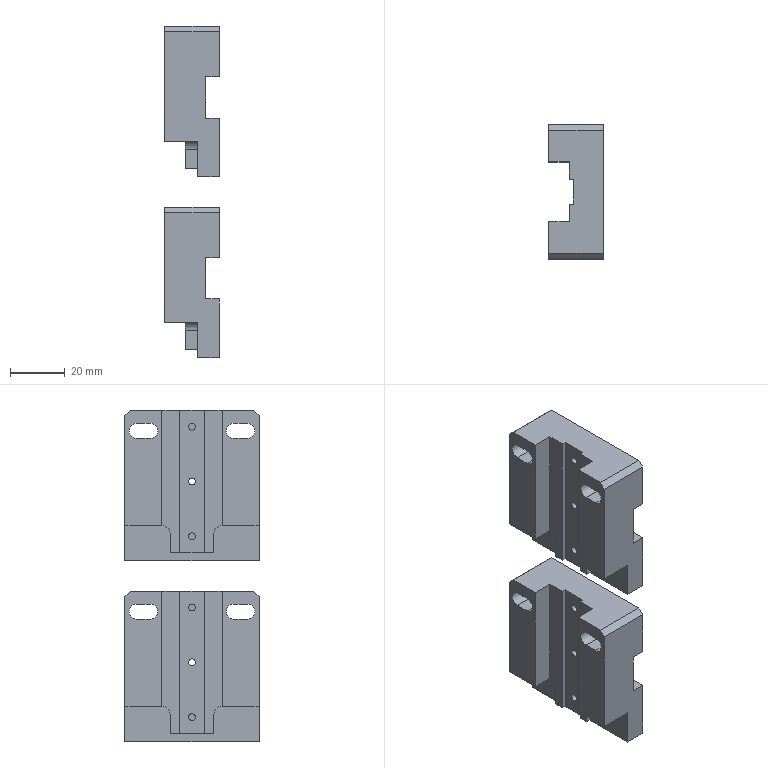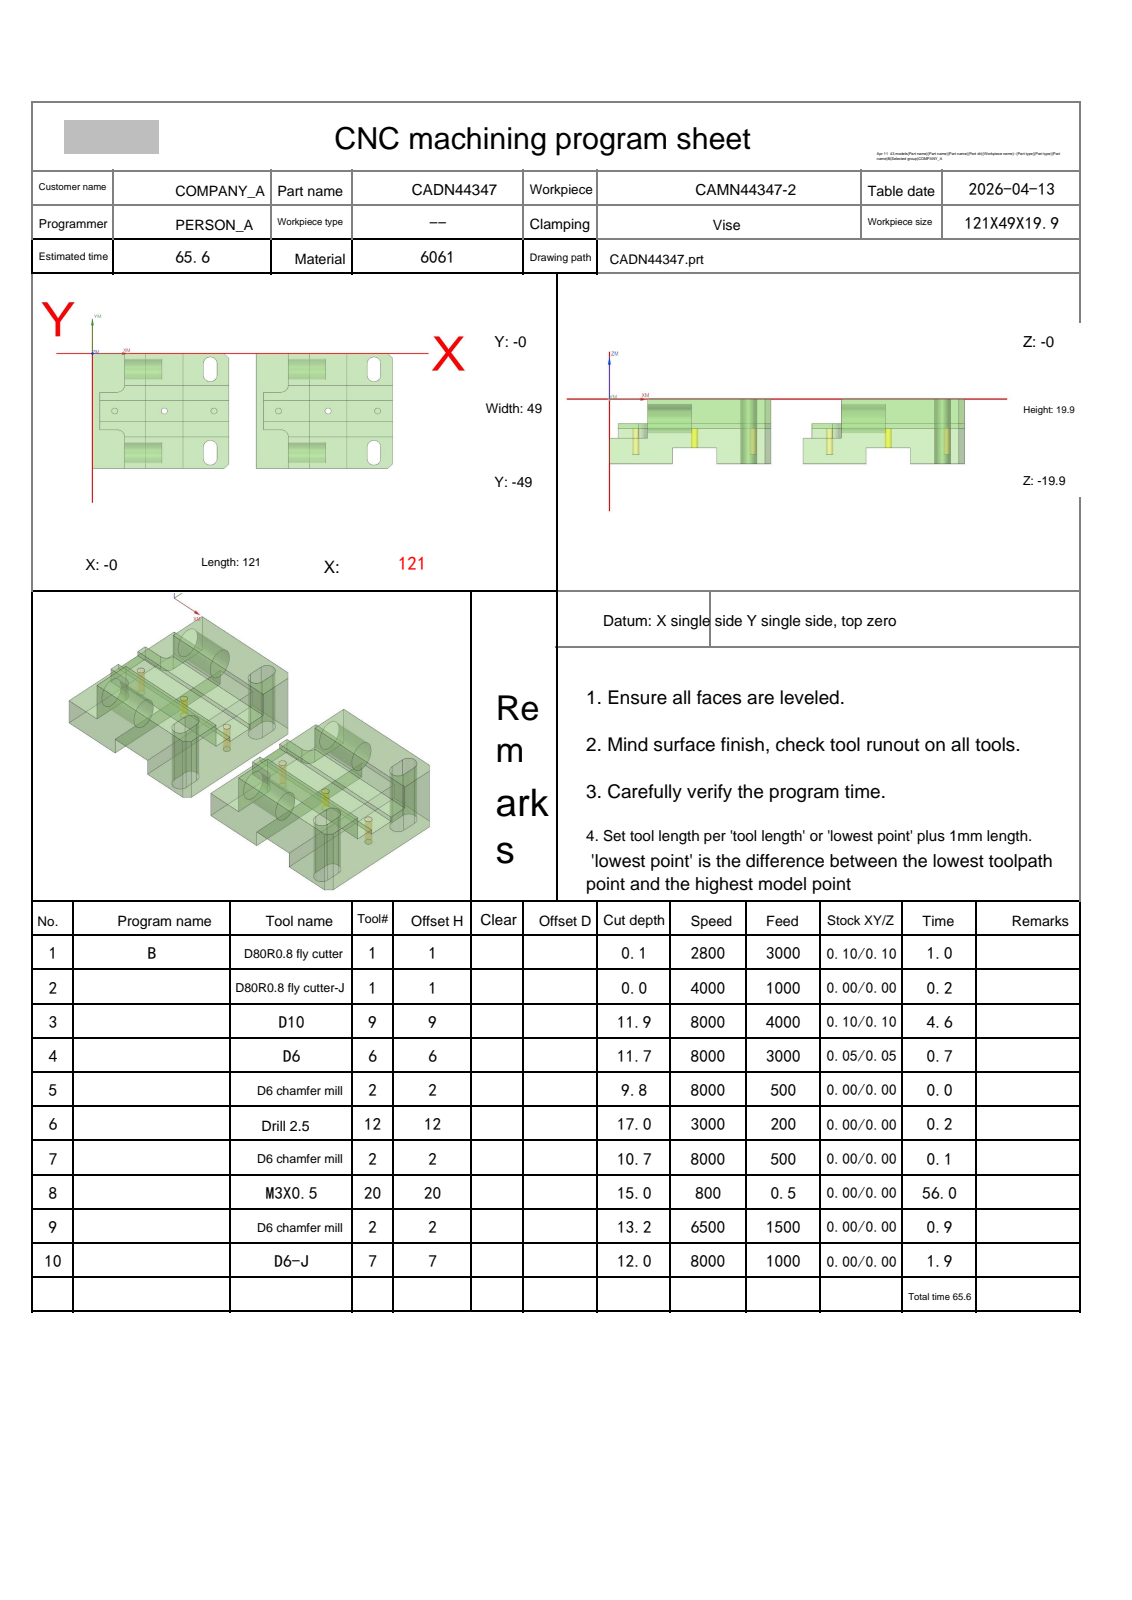NC program | NX | posted by the shop | part box 19.9 x 49 x 121 mm
Lines 120 to 1531 of 6263:
N3 T09 M06
(D10  D=10. R=0. H=09 ce=0.10 di=0.10)
G00 G90 G54 X67.5 Y-57. M03 S8000
G43 H09 Z14.902
M08
Z.905
G01 Z-.595 F4000.
Y-53.9
X61.1
Y4.9
X73.9
Y-11.4
X66.598
G02 X65.598 Y-10.4 I0.0 J1.
X65.64 Y-10.114 I1. J0.0
G01 X66.339 Y-7.77
G03 X66.38 Y-7.485 I-.958 J.285
X65.99 Y-6.693 I-1. J0.0
G02 X65.6 Y-5.902 I.61 J.793
G01 Y-.598
G02 X66.598 Y.4 I1. J-.002
G01 X68.402
G02 X69.4 Y-.598 I-.002 J-1.
G01 Y-5.902
G02 X69.038 Y-6.67 I-1. J.002
G03 X68.726 Y-7.128 I.638 J-.77
G01 X67.548 Y-10.712
G02 X66.598 Y-11.4 I-.95 J.312
G01 X63.9
Y-37.6
X73.9
Y-53.9
X70.27
G02 X69.451 Y-53.474 I0.0 J1.
G01 X66.836 Y-49.739
G03 X66.309 Y-49.357 I-.819 J-.574
G02 X65.6 Y-48.402 I.291 J.957
G01 Y-43.098
G02 X66.598 Y-42.1 I1. J-.002
G01 X68.402
G02 X69.4 Y-43.098 I-.002 J-1.
G01 Y-48.402
G02 X68.402 Y-49.4 I-1. J.002
G01 X67.5
X67.
Y-57.
Z.905
G00 X67.5
Z.31
G01 Z-1.19
Y-53.9
X61.1
Y4.9
X73.9
Y-11.4
X66.598
G02 X65.598 Y-10.4 I0.0 J1.
X65.64 Y-10.114 I1. J0.0
G01 X66.339 Y-7.77
G03 X66.38 Y-7.485 I-.958 J.285
X65.99 Y-6.693 I-1. J0.0
G02 X65.6 Y-5.902 I.61 J.793
G01 Y-.598
G02 X66.598 Y.4 I1. J-.002
G01 X68.402
G02 X69.4 Y-.598 I-.002 J-1.
G01 Y-5.902
G02 X69.038 Y-6.67 I-1. J.002
G03 X68.726 Y-7.128 I.638 J-.77
G01 X67.548 Y-10.712
G02 X66.598 Y-11.4 I-.95 J.312
G01 X63.9
Y-37.6
X73.9
Y-53.9
X70.27
G02 X69.451 Y-53.474 I0.0 J1.
G01 X66.836 Y-49.739
G03 X66.309 Y-49.357 I-.819 J-.574
G02 X65.6 Y-48.402 I.291 J.957
G01 Y-43.098
G02 X66.598 Y-42.1 I1. J-.002
G01 X68.402
G02 X69.4 Y-43.098 I-.002 J-1.
G01 Y-48.402
G02 X68.402 Y-49.4 I-1. J.002
G01 X67.5
X67.
Y-57.
Z.31
G00 X67.5
Z-.285
G01 Z-1.785
Y-53.9
X61.1
Y4.9
X73.9
Y-11.4
X66.598
G02 X65.598 Y-10.4 I0.0 J1.
X65.64 Y-10.114 I1. J0.0
G01 X66.339 Y-7.77
G03 X66.38 Y-7.485 I-.958 J.285
X65.99 Y-6.693 I-1. J0.0
G02 X65.6 Y-5.902 I.61 J.793
G01 Y-.598
G02 X66.598 Y.4 I1. J-.002
G01 X68.402
G02 X69.4 Y-.598 I-.002 J-1.
G01 Y-5.902
G02 X69.038 Y-6.67 I-1. J.002
G03 X68.726 Y-7.128 I.638 J-.77
G01 X67.548 Y-10.712
G02 X66.598 Y-11.4 I-.95 J.312
G01 X63.9
Y-37.6
X73.9
Y-53.9
X70.27
G02 X69.451 Y-53.474 I0.0 J1.
G01 X66.836 Y-49.739
G03 X66.309 Y-49.357 I-.819 J-.574
G02 X65.6 Y-48.402 I.291 J.957
G01 Y-43.098
G02 X66.598 Y-42.1 I1. J-.002
G01 X68.402
G02 X69.4 Y-43.098 I-.002 J-1.
G01 Y-48.402
G02 X68.402 Y-49.4 I-1. J.002
G01 X67.5
X67.
Y-57.
Z-.285
G00 X67.5
Z-.88
G01 Z-2.38
Y-53.9
X61.1
Y4.9
X73.9
Y-11.4
X66.598
G02 X65.598 Y-10.4 I0.0 J1.
X65.64 Y-10.114 I1. J0.0
G01 X66.339 Y-7.77
G03 X66.38 Y-7.485 I-.958 J.285
X65.99 Y-6.693 I-1. J0.0
G02 X65.6 Y-5.902 I.61 J.793
G01 Y-.598
G02 X66.598 Y.4 I1. J-.002
G01 X68.402
G02 X69.4 Y-.598 I-.002 J-1.
G01 Y-5.902
G02 X69.038 Y-6.67 I-1. J.002
G03 X68.726 Y-7.128 I.638 J-.77
G01 X67.548 Y-10.712
G02 X66.598 Y-11.4 I-.95 J.312
G01 X63.9
Y-37.6
X73.9
Y-53.9
X70.27
G02 X69.451 Y-53.474 I0.0 J1.
G01 X66.836 Y-49.739
G03 X66.309 Y-49.357 I-.819 J-.574
G02 X65.6 Y-48.402 I.291 J.957
G01 Y-43.098
G02 X66.598 Y-42.1 I1. J-.002
G01 X68.402
G02 X69.4 Y-43.098 I-.002 J-1.
G01 Y-48.402
G02 X68.402 Y-49.4 I-1. J.002
G01 X67.5
X67.
Y-57.
Z-.88
G00 X67.5
Z-1.475
G01 Z-2.975
Y-53.9
X61.1
Y4.9
X73.9
Y-11.4
X66.598
G02 X65.598 Y-10.4 I0.0 J1.
X65.64 Y-10.114 I1. J0.0
G01 X66.339 Y-7.77
G03 X66.38 Y-7.485 I-.958 J.285
X65.99 Y-6.693 I-1. J0.0
G02 X65.6 Y-5.902 I.61 J.793
G01 Y-.598
G02 X66.598 Y.4 I1. J-.002
G01 X68.402
G02 X69.4 Y-.598 I-.002 J-1.
G01 Y-5.902
G02 X69.038 Y-6.67 I-1. J.002
G03 X68.726 Y-7.128 I.638 J-.77
G01 X67.548 Y-10.712
G02 X66.598 Y-11.4 I-.95 J.312
G01 X63.9
Y-37.6
X73.9
Y-53.9
X70.27
G02 X69.451 Y-53.474 I0.0 J1.
G01 X66.836 Y-49.739
G03 X66.309 Y-49.357 I-.819 J-.574
G02 X65.6 Y-48.402 I.291 J.957
G01 Y-43.098
G02 X66.598 Y-42.1 I1. J-.002
G01 X68.402
G02 X69.4 Y-43.098 I-.002 J-1.
G01 Y-48.402
G02 X68.402 Y-49.4 I-1. J.002
G01 X67.5
X67.
Y-57.
Z-1.475
G00 X67.5
Z-2.07
G01 Z-3.57
Y-53.9
X61.1
Y4.9
X73.9
Y-11.4
X66.598
G02 X65.598 Y-10.4 I0.0 J1.
X65.64 Y-10.114 I1. J0.0
G01 X66.339 Y-7.77
G03 X66.38 Y-7.485 I-.958 J.285
X65.99 Y-6.693 I-1. J0.0
G02 X65.6 Y-5.902 I.61 J.793
G01 Y-.598
G02 X66.598 Y.4 I1. J-.002
G01 X68.402
G02 X69.4 Y-.598 I-.002 J-1.
G01 Y-5.902
G02 X69.038 Y-6.67 I-1. J.002
G03 X68.726 Y-7.128 I.638 J-.77
G01 X67.548 Y-10.712
G02 X66.598 Y-11.4 I-.95 J.312
G01 X63.9
Y-37.6
X73.9
Y-53.9
X70.27
G02 X69.451 Y-53.474 I0.0 J1.
G01 X66.836 Y-49.739
G03 X66.309 Y-49.357 I-.819 J-.574
G02 X65.6 Y-48.402 I.291 J.957
G01 Y-43.098
G02 X66.598 Y-42.1 I1. J-.002
G01 X68.402
G02 X69.4 Y-43.098 I-.002 J-1.
G01 Y-48.402
G02 X68.402 Y-49.4 I-1. J.002
G01 X67.5
X67.
Y-57.
Z-2.07
G00 X67.5
Z-2.665
G01 Z-4.165
Y-53.9
X61.1
Y4.9
X73.9
Y-11.4
X66.598
G02 X65.598 Y-10.4 I0.0 J1.
X65.64 Y-10.114 I1. J0.0
G01 X66.339 Y-7.77
G03 X66.38 Y-7.485 I-.958 J.285
X65.99 Y-6.693 I-1. J0.0
G02 X65.6 Y-5.902 I.61 J.793
G01 Y-.598
G02 X66.598 Y.4 I1. J-.002
G01 X68.402
G02 X69.4 Y-.598 I-.002 J-1.
G01 Y-5.902
G02 X69.038 Y-6.67 I-1. J.002
G03 X68.726 Y-7.128 I.638 J-.77
G01 X67.548 Y-10.712
G02 X66.598 Y-11.4 I-.95 J.312
G01 X63.9
Y-37.6
X73.9
Y-53.9
X70.27
G02 X69.451 Y-53.474 I0.0 J1.
G01 X66.836 Y-49.739
G03 X66.309 Y-49.357 I-.819 J-.574
G02 X65.6 Y-48.402 I.291 J.957
G01 Y-43.098
G02 X66.598 Y-42.1 I1. J-.002
G01 X68.402
G02 X69.4 Y-43.098 I-.002 J-1.
G01 Y-48.402
G02 X68.402 Y-49.4 I-1. J.002
G01 X67.5
X67.
Y-57.
Z-2.665
G00 X67.5
Z-3.26
G01 Z-4.76
Y-53.9
X61.1
Y4.9
X73.9
Y-11.4
X66.598
G02 X65.598 Y-10.4 I0.0 J1.
X65.64 Y-10.114 I1. J0.0
G01 X66.339 Y-7.77
G03 X66.38 Y-7.485 I-.958 J.285
X65.99 Y-6.693 I-1. J0.0
G02 X65.6 Y-5.902 I.61 J.793
G01 Y-.598
G02 X66.598 Y.4 I1. J-.002
G01 X68.402
G02 X69.4 Y-.598 I-.002 J-1.
G01 Y-5.902
G02 X69.038 Y-6.67 I-1. J.002
G03 X68.726 Y-7.128 I.638 J-.77
G01 X67.548 Y-10.712
G02 X66.598 Y-11.4 I-.95 J.312
G01 X63.9
Y-37.6
X73.9
Y-53.9
X70.27
G02 X69.451 Y-53.474 I0.0 J1.
G01 X66.836 Y-49.739
G03 X66.309 Y-49.357 I-.819 J-.574
G02 X65.6 Y-48.402 I.291 J.957
G01 Y-43.098
G02 X66.598 Y-42.1 I1. J-.002
G01 X68.402
G02 X69.4 Y-43.098 I-.002 J-1.
G01 Y-48.402
G02 X68.402 Y-49.4 I-1. J.002
G01 X67.5
X67.
Y-57.
Z-3.26
G00 X67.5
Z-3.855
G01 Z-5.355
Y-53.9
X61.1
Y4.9
X73.9
Y-11.4
X66.598
G02 X65.598 Y-10.4 I0.0 J1.
X65.64 Y-10.114 I1. J0.0
G01 X66.339 Y-7.77
G03 X66.38 Y-7.485 I-.958 J.285
X65.99 Y-6.693 I-1. J0.0
G02 X65.6 Y-5.902 I.61 J.793
G01 Y-.598
G02 X66.598 Y.4 I1. J-.002
G01 X68.402
G02 X69.4 Y-.598 I-.002 J-1.
G01 Y-5.902
G02 X69.038 Y-6.67 I-1. J.002
G03 X68.726 Y-7.128 I.638 J-.77
G01 X67.548 Y-10.712
G02 X66.598 Y-11.4 I-.95 J.312
G01 X63.9
Y-37.6
X73.9
Y-53.9
X70.27
G02 X69.451 Y-53.474 I0.0 J1.
G01 X66.836 Y-49.739
G03 X66.309 Y-49.357 I-.819 J-.574
G02 X65.6 Y-48.402 I.291 J.957
G01 Y-43.098
G02 X66.598 Y-42.1 I1. J-.002
G01 X68.402
G02 X69.4 Y-43.098 I-.002 J-1.
G01 Y-48.402
G02 X68.402 Y-49.4 I-1. J.002
G01 X67.5
X67.
Y-57.
Z-3.855
G00 X67.5
Z-4.45
G01 Z-5.95
Y-53.9
X61.1
Y4.9
X73.9
Y-11.4
X66.598
G02 X65.598 Y-10.4 I0.0 J1.
X65.64 Y-10.114 I1. J0.0
G01 X66.339 Y-7.77
G03 X66.38 Y-7.485 I-.958 J.285
X65.99 Y-6.693 I-1. J0.0
G02 X65.6 Y-5.902 I.61 J.793
G01 Y-.598
G02 X66.598 Y.4 I1. J-.002
G01 X68.402
G02 X69.4 Y-.598 I-.002 J-1.
G01 Y-5.902
G02 X69.038 Y-6.67 I-1. J.002
G03 X68.726 Y-7.128 I.638 J-.77
G01 X67.548 Y-10.712
G02 X66.598 Y-11.4 I-.95 J.312
G01 X63.9
Y-37.6
X73.9
Y-53.9
X70.27
G02 X69.451 Y-53.474 I0.0 J1.
G01 X66.836 Y-49.739
G03 X66.309 Y-49.357 I-.819 J-.574
G02 X65.6 Y-48.402 I.291 J.957
G01 Y-43.098
G02 X66.598 Y-42.1 I1. J-.002
G01 X68.402
G02 X69.4 Y-43.098 I-.002 J-1.
G01 Y-48.402
G02 X68.402 Y-49.4 I-1. J.002
G01 X67.5
X67.
Y-57.
Z-4.45
G00 X67.5
Z-5.045
G01 Z-6.545
Y-53.9
X61.1
Y4.9
X73.9
Y-11.4
X66.598
G02 X65.598 Y-10.4 I0.0 J1.
X65.64 Y-10.114 I1. J0.0
G01 X66.339 Y-7.77
G03 X66.38 Y-7.485 I-.958 J.285
X65.99 Y-6.693 I-1. J0.0
G02 X65.6 Y-5.902 I.61 J.793
G01 Y-.598
G02 X66.598 Y.4 I1. J-.002
G01 X68.402
G02 X69.4 Y-.598 I-.002 J-1.
G01 Y-5.902
G02 X69.038 Y-6.67 I-1. J.002
G03 X68.726 Y-7.128 I.638 J-.77
G01 X67.548 Y-10.712
G02 X66.598 Y-11.4 I-.95 J.312
G01 X63.9
Y-37.6
X73.9
Y-53.9
X70.27
G02 X69.451 Y-53.474 I0.0 J1.
G01 X66.836 Y-49.739
G03 X66.309 Y-49.357 I-.819 J-.574
G02 X65.6 Y-48.402 I.291 J.957
G01 Y-43.098
G02 X66.598 Y-42.1 I1. J-.002
G01 X68.402
G02 X69.4 Y-43.098 I-.002 J-1.
G01 Y-48.402
G02 X68.402 Y-49.4 I-1. J.002
G01 X67.5
X67.
Y-57.
Z-5.045
G00 X67.5
Z-5.64
G01 Z-7.14
Y-53.9
X61.1
Y4.9
X73.9
Y-11.4
X66.598
G02 X65.598 Y-10.4 I0.0 J1.
X65.64 Y-10.114 I1. J0.0
G01 X66.339 Y-7.77
G03 X66.38 Y-7.485 I-.958 J.285
X65.99 Y-6.693 I-1. J0.0
G02 X65.6 Y-5.902 I.61 J.793
G01 Y-.598
G02 X66.598 Y.4 I1. J-.002
G01 X68.402
G02 X69.4 Y-.598 I-.002 J-1.
G01 Y-5.902
G02 X69.038 Y-6.67 I-1. J.002
G03 X68.726 Y-7.128 I.638 J-.77
G01 X67.548 Y-10.712
G02 X66.598 Y-11.4 I-.95 J.312
G01 X63.9
Y-37.6
X73.9
Y-53.9
X70.27
G02 X69.451 Y-53.474 I0.0 J1.
G01 X66.836 Y-49.739
G03 X66.309 Y-49.357 I-.819 J-.574
G02 X65.6 Y-48.402 I.291 J.957
G01 Y-43.098
G02 X66.598 Y-42.1 I1. J-.002
G01 X68.402
G02 X69.4 Y-43.098 I-.002 J-1.
G01 Y-48.402
G02 X68.402 Y-49.4 I-1. J.002
G01 X67.5
X67.
Y-57.
Z-5.64
G00 X67.5
Z-6.235
G01 Z-7.735
Y-53.9
X61.1
Y4.9
X73.9
Y-11.4
X66.598
G02 X65.598 Y-10.4 I0.0 J1.
X65.64 Y-10.114 I1. J0.0
G01 X66.339 Y-7.77
G03 X66.38 Y-7.485 I-.958 J.285
X65.99 Y-6.693 I-1. J0.0
G02 X65.6 Y-5.902 I.61 J.793
G01 Y-.598
G02 X66.598 Y.4 I1. J-.002
G01 X68.402
G02 X69.4 Y-.598 I-.002 J-1.
G01 Y-5.902
G02 X69.038 Y-6.67 I-1. J.002
G03 X68.726 Y-7.128 I.638 J-.77
G01 X67.548 Y-10.712
G02 X66.598 Y-11.4 I-.95 J.312
G01 X63.9
Y-37.6
X73.9
Y-53.9
X70.27
G02 X69.451 Y-53.474 I0.0 J1.
G01 X66.836 Y-49.739
G03 X66.309 Y-49.357 I-.819 J-.574
G02 X65.6 Y-48.402 I.291 J.957
G01 Y-43.098
G02 X66.598 Y-42.1 I1. J-.002
G01 X68.402
G02 X69.4 Y-43.098 I-.002 J-1.
G01 Y-48.402
G02 X68.402 Y-49.4 I-1. J.002
G01 X67.5
X67.
Y-57.
Z-6.235
G00 X67.5
Z-6.83
G01 Z-8.33
Y-53.9
X61.1
Y4.9
X73.9
Y-11.4
X66.598
G02 X65.598 Y-10.4 I0.0 J1.
X65.64 Y-10.114 I1. J0.0
G01 X66.339 Y-7.77
G03 X66.38 Y-7.485 I-.958 J.285
X65.99 Y-6.693 I-1. J0.0
G02 X65.6 Y-5.902 I.61 J.793
G01 Y-.598
G02 X66.598 Y.4 I1. J-.002
G01 X68.402
G02 X69.4 Y-.598 I-.002 J-1.
G01 Y-5.902
G02 X69.038 Y-6.67 I-1. J.002
G03 X68.726 Y-7.128 I.638 J-.77
G01 X67.548 Y-10.712
G02 X66.598 Y-11.4 I-.95 J.312
G01 X63.9
Y-37.6
X73.9
Y-53.9
X70.27
G02 X69.451 Y-53.474 I0.0 J1.
G01 X66.836 Y-49.739
G03 X66.309 Y-49.357 I-.819 J-.574
G02 X65.6 Y-48.402 I.291 J.957
G01 Y-43.098
G02 X66.598 Y-42.1 I1. J-.002
G01 X68.402
G02 X69.4 Y-43.098 I-.002 J-1.
G01 Y-48.402
G02 X68.402 Y-49.4 I-1. J.002
G01 X67.5
X67.
Y-57.
Z-6.83
G00 X67.5
Z-7.425
G01 Z-8.925
Y-53.9
X61.1
Y4.9
X73.9
Y-11.4
X66.598
G02 X65.598 Y-10.4 I0.0 J1.
X65.64 Y-10.114 I1. J0.0
G01 X66.339 Y-7.77
G03 X66.38 Y-7.485 I-.958 J.285
X65.99 Y-6.693 I-1. J0.0
G02 X65.6 Y-5.902 I.61 J.793
G01 Y-.598
G02 X66.598 Y.4 I1. J-.002
G01 X68.402
G02 X69.4 Y-.598 I-.002 J-1.
G01 Y-5.902
G02 X69.038 Y-6.67 I-1. J.002
G03 X68.726 Y-7.128 I.638 J-.77
G01 X67.548 Y-10.712
G02 X66.598 Y-11.4 I-.95 J.312
G01 X63.9
Y-37.6
X73.9
Y-53.9
X70.27
G02 X69.451 Y-53.474 I0.0 J1.
G01 X66.836 Y-49.739
G03 X66.309 Y-49.357 I-.819 J-.574
G02 X65.6 Y-48.402 I.291 J.957
G01 Y-43.098
G02 X66.598 Y-42.1 I1. J-.002
G01 X68.402
G02 X69.4 Y-43.098 I-.002 J-1.
G01 Y-48.402
G02 X68.402 Y-49.4 I-1. J.002
G01 X67.5
X67.
Y-57.
Z-7.425
G00 X67.5
Z-8.02
G01 Z-9.52
Y-53.9
X61.1
Y4.9
X73.9
Y-11.4
X66.598
G02 X65.598 Y-10.4 I0.0 J1.
X65.64 Y-10.114 I1. J0.0
G01 X66.339 Y-7.77
G03 X66.38 Y-7.485 I-.958 J.285
X65.99 Y-6.693 I-1. J0.0
G02 X65.6 Y-5.902 I.61 J.793
G01 Y-.598
G02 X66.598 Y.4 I1. J-.002
G01 X68.402
G02 X69.4 Y-.598 I-.002 J-1.
G01 Y-5.902
G02 X69.038 Y-6.67 I-1. J.002
G03 X68.726 Y-7.128 I.638 J-.77
G01 X67.548 Y-10.712
G02 X66.598 Y-11.4 I-.95 J.312
G01 X63.9
Y-37.6
X73.9
Y-53.9
X70.27
G02 X69.451 Y-53.474 I0.0 J1.
G01 X66.836 Y-49.739
G03 X66.309 Y-49.357 I-.819 J-.574
G02 X65.6 Y-48.402 I.291 J.957
G01 Y-43.098
G02 X66.598 Y-42.1 I1. J-.002
G01 X68.402
G02 X69.4 Y-43.098 I-.002 J-1.
G01 Y-48.402
G02 X68.402 Y-49.4 I-1. J.002
G01 X67.5
X67.
Y-57.
Z-8.02
G00 X67.5
Z-8.615
G01 Z-10.115
Y-53.9
X61.1
Y4.9
X73.9
Y-11.4
X66.598
G02 X65.598 Y-10.4 I0.0 J1.
X65.64 Y-10.114 I1. J0.0
G01 X66.339 Y-7.77
G03 X66.38 Y-7.485 I-.958 J.285
X65.99 Y-6.693 I-1. J0.0
G02 X65.6 Y-5.902 I.61 J.793
G01 Y-.598
G02 X66.598 Y.4 I1. J-.002
G01 X68.402
G02 X69.4 Y-.598 I-.002 J-1.
G01 Y-5.902
G02 X69.038 Y-6.67 I-1. J.002
G03 X68.726 Y-7.128 I.638 J-.77
G01 X67.548 Y-10.712
G02 X66.598 Y-11.4 I-.95 J.312
G01 X63.9
Y-37.6
X73.9
Y-53.9
X70.27
G02 X69.451 Y-53.474 I0.0 J1.
G01 X66.836 Y-49.739
G03 X66.309 Y-49.357 I-.819 J-.574
G02 X65.6 Y-48.402 I.291 J.957
G01 Y-43.098
G02 X66.598 Y-42.1 I1. J-.002
G01 X68.402
G02 X69.4 Y-43.098 I-.002 J-1.
G01 Y-48.402
G02 X68.402 Y-49.4 I-1. J.002
G01 X67.5
X67.
Y-57.
Z-8.615
G00 X67.5
Z-9.21
G01 Z-10.71
Y-53.9
X61.1
Y4.9
X73.9
Y-11.4
X66.598
G02 X65.598 Y-10.4 I0.0 J1.
X65.64 Y-10.114 I1. J0.0
G01 X66.339 Y-7.77
G03 X66.38 Y-7.485 I-.958 J.285
X65.99 Y-6.693 I-1. J0.0
G02 X65.6 Y-5.902 I.61 J.793
G01 Y-.598
G02 X66.598 Y.4 I1. J-.002
G01 X68.402
G02 X69.4 Y-.598 I-.002 J-1.
G01 Y-5.902
G02 X69.038 Y-6.67 I-1. J.002
G03 X68.726 Y-7.128 I.638 J-.77
G01 X67.548 Y-10.712
G02 X66.598 Y-11.4 I-.95 J.312
G01 X63.9
Y-37.6
X73.9
Y-53.9
X70.27
G02 X69.451 Y-53.474 I0.0 J1.
G01 X66.836 Y-49.739
G03 X66.309 Y-49.357 I-.819 J-.574
G02 X65.6 Y-48.402 I.291 J.957
G01 Y-43.098
G02 X66.598 Y-42.1 I1. J-.002
G01 X68.402
G02 X69.4 Y-43.098 I-.002 J-1.
G01 Y-48.402
G02 X68.402 Y-49.4 I-1. J.002
G01 X67.5
X67.
Y-57.
Z-9.21
G00 X67.5
Z-9.805
G01 Z-11.305
Y-53.9
X61.1
Y4.9
X73.9
Y-11.4
X66.598
G02 X65.598 Y-10.4 I0.0 J1.
X65.64 Y-10.114 I1. J0.0
G01 X66.339 Y-7.77
G03 X66.38 Y-7.485 I-.958 J.285
X65.99 Y-6.693 I-1. J0.0
G02 X65.6 Y-5.902 I.61 J.793
G01 Y-.598
G02 X66.598 Y.4 I1. J-.002
G01 X68.402
G02 X69.4 Y-.598 I-.002 J-1.
G01 Y-5.902
G02 X69.038 Y-6.67 I-1. J.002
G03 X68.726 Y-7.128 I.638 J-.77
G01 X67.548 Y-10.712
G02 X66.598 Y-11.4 I-.95 J.312
G01 X63.9
Y-37.6
X73.9
Y-53.9
X70.27
G02 X69.451 Y-53.474 I0.0 J1.
G01 X66.836 Y-49.739
G03 X66.309 Y-49.357 I-.819 J-.574
G02 X65.6 Y-48.402 I.291 J.957
G01 Y-43.098
G02 X66.598 Y-42.1 I1. J-.002
G01 X68.402
G02 X69.4 Y-43.098 I-.002 J-1.
G01 Y-48.402
G02 X68.402 Y-49.4 I-1. J.002
G01 X67.5
X67.
Y-57.
Z-9.805
G00 X67.5
Z-10.4
G01 Z-11.9
Y-53.9
X61.1
Y4.9
X73.9
Y-11.4
X66.598
G02 X65.598 Y-10.4 I0.0 J1.
X65.64 Y-10.114 I1. J0.0
G01 X66.339 Y-7.77
G03 X66.38 Y-7.485 I-.958 J.285
X65.99 Y-6.693 I-1. J0.0
G02 X65.6 Y-5.902 I.61 J.793
G01 Y-.598
G02 X66.598 Y.4 I1. J-.002
G01 X68.402
G02 X69.4 Y-.598 I-.002 J-1.
G01 Y-5.902
G02 X69.038 Y-6.67 I-1. J.002
G03 X68.726 Y-7.128 I.638 J-.77
G01 X67.548 Y-10.712
G02 X66.598 Y-11.4 I-.95 J.312
G01 X63.9
Y-37.6
X73.9
Y-53.9
X70.27
G02 X69.451 Y-53.474 I0.0 J1.
G01 X66.836 Y-49.739
G03 X66.309 Y-49.357 I-.819 J-.574
G02 X65.6 Y-48.402 I.291 J.957
G01 Y-43.098
G02 X66.598 Y-42.1 I1. J-.002
G01 X68.402
G02 X69.4 Y-43.098 I-.002 J-1.
G01 Y-48.402
G02 X68.402 Y-49.4 I-1. J.002
G01 X67.5
X67.
Y-57.
Z-10.4
G00 Z14.902
X-8. Y-45.75
Z.905
G01 Z-.595
X-4.9
Y4.9
X7.9
Y-11.4
X.598
G02 X-.402 Y-10.4 I0.0 J1.
X-.36 Y-10.114 I1. J0.0
G01 X.339 Y-7.77
G03 X.38 Y-7.485 I-.958 J.285
X-.01 Y-6.693 I-1. J0.0
G02 X-.4 Y-5.902 I.61 J.793
G01 Y-.598
G02 X.598 Y.4 I1. J-.002
G01 X2.402
G02 X3.4 Y-.598 I-.002 J-1.
G01 Y-5.902
G02 X3.038 Y-6.67 I-1. J.002
G03 X2.726 Y-7.128 I.638 J-.77
G01 X1.548 Y-10.712
G02 X.598 Y-11.4 I-.95 J.312
G01 X-2.1
Y-37.6
X7.9
Y-53.9
X-4.9
Y-48.414
G02 X-4.607 Y-47.707 I1. J0.0
G01 X-.693 Y-43.793
G03 X-.4 Y-43.093 I-.707 J.707
G02 X.598 Y-42.1 I1. J-.007
G01 X2.402
G02 X3.4 Y-43.098 I-.002 J-1.
G01 Y-48.402
G02 X2.402 Y-49.4 I-1. J.002
G01 X.598
G02 X-.4 Y-48.402 I.002 J1.
G01 Y-45.75
Y-45.25
X-8.
Z.905
G00 Y-45.75
Z.31
G01 Z-1.19
X-4.9
Y4.9
X7.9
Y-11.4
X.598
G02 X-.402 Y-10.4 I0.0 J1.
X-.36 Y-10.114 I1. J0.0
G01 X.339 Y-7.77
G03 X.38 Y-7.485 I-.958 J.285
X-.01 Y-6.693 I-1. J0.0
G02 X-.4 Y-5.902 I.61 J.793
G01 Y-.598
G02 X.598 Y.4 I1. J-.002
G01 X2.402
G02 X3.4 Y-.598 I-.002 J-1.
G01 Y-5.902
G02 X3.038 Y-6.67 I-1. J.002
G03 X2.726 Y-7.128 I.638 J-.77
G01 X1.548 Y-10.712
G02 X.598 Y-11.4 I-.95 J.312
G01 X-2.1
Y-37.6
X7.9
Y-53.9
X-4.9
Y-48.414
G02 X-4.607 Y-47.707 I1. J0.0
G01 X-.693 Y-43.793
G03 X-.4 Y-43.093 I-.707 J.707
G02 X.598 Y-42.1 I1. J-.007
G01 X2.402
G02 X3.4 Y-43.098 I-.002 J-1.
G01 Y-48.402
G02 X2.402 Y-49.4 I-1. J.002
G01 X.598
G02 X-.4 Y-48.402 I.002 J1.
G01 Y-45.75
Y-45.25
X-8.
Z.31
G00 Y-45.75
Z-.285
G01 Z-1.785
X-4.9
Y4.9
X7.9
Y-11.4
X.598
G02 X-.402 Y-10.4 I0.0 J1.
X-.36 Y-10.114 I1. J0.0
G01 X.339 Y-7.77
G03 X.38 Y-7.485 I-.958 J.285
X-.01 Y-6.693 I-1. J0.0
G02 X-.4 Y-5.902 I.61 J.793
G01 Y-.598
G02 X.598 Y.4 I1. J-.002
G01 X2.402
G02 X3.4 Y-.598 I-.002 J-1.
G01 Y-5.902
G02 X3.038 Y-6.67 I-1. J.002
G03 X2.726 Y-7.128 I.638 J-.77
G01 X1.548 Y-10.712
G02 X.598 Y-11.4 I-.95 J.312
G01 X-2.1
Y-37.6
X7.9
Y-53.9
X-4.9
Y-48.414
G02 X-4.607 Y-47.707 I1. J0.0
G01 X-.693 Y-43.793
G03 X-.4 Y-43.093 I-.707 J.707
G02 X.598 Y-42.1 I1. J-.007
G01 X2.402
G02 X3.4 Y-43.098 I-.002 J-1.
G01 Y-48.402
G02 X2.402 Y-49.4 I-1. J.002
G01 X.598
G02 X-.4 Y-48.402 I.002 J1.
G01 Y-45.75
Y-45.25
X-8.
Z-.285
G00 Y-45.75
Z-.88
G01 Z-2.38
X-4.9
Y4.9
X7.9
Y-11.4
X.598
G02 X-.402 Y-10.4 I0.0 J1.
X-.36 Y-10.114 I1. J0.0
G01 X.339 Y-7.77
G03 X.38 Y-7.485 I-.958 J.285
X-.01 Y-6.693 I-1. J0.0
G02 X-.4 Y-5.902 I.61 J.793
G01 Y-.598
G02 X.598 Y.4 I1. J-.002
G01 X2.402
G02 X3.4 Y-.598 I-.002 J-1.
G01 Y-5.902
G02 X3.038 Y-6.67 I-1. J.002
G03 X2.726 Y-7.128 I.638 J-.77
G01 X1.548 Y-10.712
G02 X.598 Y-11.4 I-.95 J.312
G01 X-2.1
Y-37.6
X7.9
Y-53.9
X-4.9
Y-48.414
G02 X-4.607 Y-47.707 I1. J0.0
G01 X-.693 Y-43.793
G03 X-.4 Y-43.093 I-.707 J.707
G02 X.598 Y-42.1 I1. J-.007
G01 X2.402
G02 X3.4 Y-43.098 I-.002 J-1.
G01 Y-48.402
G02 X2.402 Y-49.4 I-1. J.002
G01 X.598
G02 X-.4 Y-48.402 I.002 J1.
G01 Y-45.75
Y-45.25
X-8.
Z-.88
G00 Y-45.75
Z-1.475
G01 Z-2.975
X-4.9
Y4.9
X7.9
Y-11.4
X.598
G02 X-.402 Y-10.4 I0.0 J1.
X-.36 Y-10.114 I1. J0.0
G01 X.339 Y-7.77
G03 X.38 Y-7.485 I-.958 J.285
X-.01 Y-6.693 I-1. J0.0
G02 X-.4 Y-5.902 I.61 J.793
G01 Y-.598
G02 X.598 Y.4 I1. J-.002
G01 X2.402
G02 X3.4 Y-.598 I-.002 J-1.
G01 Y-5.902
G02 X3.038 Y-6.67 I-1. J.002
G03 X2.726 Y-7.128 I.638 J-.77
G01 X1.548 Y-10.712
G02 X.598 Y-11.4 I-.95 J.312
G01 X-2.1
Y-37.6
X7.9
Y-53.9
X-4.9
Y-48.414
G02 X-4.607 Y-47.707 I1. J0.0
G01 X-.693 Y-43.793
G03 X-.4 Y-43.093 I-.707 J.707
G02 X.598 Y-42.1 I1. J-.007
G01 X2.402
G02 X3.4 Y-43.098 I-.002 J-1.
G01 Y-48.402
G02 X2.402 Y-49.4 I-1. J.002
G01 X.598
G02 X-.4 Y-48.402 I.002 J1.
G01 Y-45.75
Y-45.25
X-8.
Z-1.475
G00 Y-45.75
Z-2.07
G01 Z-3.57
X-4.9
Y4.9
X7.9
Y-11.4
X.598
G02 X-.402 Y-10.4 I0.0 J1.
X-.36 Y-10.114 I1. J0.0
G01 X.339 Y-7.77
G03 X.38 Y-7.485 I-.958 J.285
X-.01 Y-6.693 I-1. J0.0
G02 X-.4 Y-5.902 I.61 J.793
G01 Y-.598
G02 X.598 Y.4 I1. J-.002
G01 X2.402
G02 X3.4 Y-.598 I-.002 J-1.
G01 Y-5.902
G02 X3.038 Y-6.67 I-1. J.002
G03 X2.726 Y-7.128 I.638 J-.77
G01 X1.548 Y-10.712
G02 X.598 Y-11.4 I-.95 J.312
G01 X-2.1
Y-37.6
X7.9
Y-53.9
X-4.9
Y-48.414
G02 X-4.607 Y-47.707 I1. J0.0
G01 X-.693 Y-43.793
G03 X-.4 Y-43.093 I-.707 J.707
G02 X.598 Y-42.1 I1. J-.007
G01 X2.402
G02 X3.4 Y-43.098 I-.002 J-1.
G01 Y-48.402
G02 X2.402 Y-49.4 I-1. J.002
G01 X.598
G02 X-.4 Y-48.402 I.002 J1.
G01 Y-45.75
Y-45.25
X-8.
Z-2.07
G00 Y-45.75
Z-2.665
G01 Z-4.165
X-4.9
Y4.9
X7.9
Y-11.4
X.598
G02 X-.402 Y-10.4 I0.0 J1.
X-.36 Y-10.114 I1. J0.0
G01 X.339 Y-7.77
G03 X.38 Y-7.485 I-.958 J.285
X-.01 Y-6.693 I-1. J0.0
G02 X-.4 Y-5.902 I.61 J.793
G01 Y-.598
G02 X.598 Y.4 I1. J-.002
G01 X2.402
G02 X3.4 Y-.598 I-.002 J-1.
G01 Y-5.902
G02 X3.038 Y-6.67 I-1. J.002
G03 X2.726 Y-7.128 I.638 J-.77
G01 X1.548 Y-10.712
G02 X.598 Y-11.4 I-.95 J.312
G01 X-2.1
Y-37.6
X7.9
Y-53.9
X-4.9
Y-48.414
G02 X-4.607 Y-47.707 I1. J0.0
G01 X-.693 Y-43.793
G03 X-.4 Y-43.093 I-.707 J.707
G02 X.598 Y-42.1 I1. J-.007
G01 X2.402
G02 X3.4 Y-43.098 I-.002 J-1.
G01 Y-48.402
G02 X2.402 Y-49.4 I-1. J.002
G01 X.598
G02 X-.4 Y-48.402 I.002 J1.
G01 Y-45.75
Y-45.25
X-8.
Z-2.665
G00 Y-45.75
Z-3.26
G01 Z-4.76
X-4.9
Y4.9
X7.9
Y-11.4
X.598
G02 X-.402 Y-10.4 I0.0 J1.
X-.36 Y-10.114 I1. J0.0
G01 X.339 Y-7.77
G03 X.38 Y-7.485 I-.958 J.285
X-.01 Y-6.693 I-1. J0.0
G02 X-.4 Y-5.902 I.61 J.793
G01 Y-.598
G02 X.598 Y.4 I1. J-.002
G01 X2.402
G02 X3.4 Y-.598 I-.002 J-1.
G01 Y-5.902
G02 X3.038 Y-6.67 I-1. J.002
G03 X2.726 Y-7.128 I.638 J-.77
G01 X1.548 Y-10.712
G02 X.598 Y-11.4 I-.95 J.312
G01 X-2.1
Y-37.6
X7.9
Y-53.9
X-4.9
Y-48.414
G02 X-4.607 Y-47.707 I1. J0.0
G01 X-.693 Y-43.793
G03 X-.4 Y-43.093 I-.707 J.707
G02 X.598 Y-42.1 I1. J-.007
G01 X2.402
G02 X3.4 Y-43.098 I-.002 J-1.
G01 Y-48.402
G02 X2.402 Y-49.4 I-1. J.002
G01 X.598
G02 X-.4 Y-48.402 I.002 J1.
G01 Y-45.75
Y-45.25
X-8.
Z-3.26
G00 Y-45.75
Z-3.855
G01 Z-5.355
X-4.9
Y4.9
X7.9
Y-11.4
X.598
G02 X-.402 Y-10.4 I0.0 J1.
X-.36 Y-10.114 I1. J0.0
G01 X.339 Y-7.77
G03 X.38 Y-7.485 I-.958 J.285
X-.01 Y-6.693 I-1. J0.0
G02 X-.4 Y-5.902 I.61 J.793
G01 Y-.598
G02 X.598 Y.4 I1. J-.002
G01 X2.402
G02 X3.4 Y-.598 I-.002 J-1.
G01 Y-5.902
G02 X3.038 Y-6.67 I-1. J.002
G03 X2.726 Y-7.128 I.638 J-.77
G01 X1.548 Y-10.712
G02 X.598 Y-11.4 I-.95 J.312
G01 X-2.1
Y-37.6
X7.9
Y-53.9
X-4.9
Y-48.414
G02 X-4.607 Y-47.707 I1. J0.0
G01 X-.693 Y-43.793
G03 X-.4 Y-43.093 I-.707 J.707
G02 X.598 Y-42.1 I1. J-.007
G01 X2.402
G02 X3.4 Y-43.098 I-.002 J-1.
G01 Y-48.402
G02 X2.402 Y-49.4 I-1. J.002
G01 X.598
G02 X-.4 Y-48.402 I.002 J1.
G01 Y-45.75
Y-45.25
X-8.
Z-3.855
G00 Y-45.75
Z-4.45
G01 Z-5.95
X-4.9
Y4.9
X7.9
Y-11.4
X.598
G02 X-.402 Y-10.4 I0.0 J1.
X-.36 Y-10.114 I1. J0.0
G01 X.339 Y-7.77
G03 X.38 Y-7.485 I-.958 J.285
X-.01 Y-6.693 I-1. J0.0
G02 X-.4 Y-5.902 I.61 J.793
G01 Y-.598
G02 X.598 Y.4 I1. J-.002
G01 X2.402
G02 X3.4 Y-.598 I-.002 J-1.
G01 Y-5.902
G02 X3.038 Y-6.67 I-1. J.002
G03 X2.726 Y-7.128 I.638 J-.77
G01 X1.548 Y-10.712
G02 X.598 Y-11.4 I-.95 J.312
G01 X-2.1
Y-37.6
X7.9
Y-53.9
X-4.9
Y-48.414
G02 X-4.607 Y-47.707 I1. J0.0
G01 X-.693 Y-43.793
G03 X-.4 Y-43.093 I-.707 J.707
G02 X.598 Y-42.1 I1. J-.007
G01 X2.402
G02 X3.4 Y-43.098 I-.002 J-1.
G01 Y-48.402
G02 X2.402 Y-49.4 I-1. J.002
G01 X.598
G02 X-.4 Y-48.402 I.002 J1.
G01 Y-45.75
Y-45.25
X-8.
Z-4.45
G00 Y-45.75
Z-5.045
G01 Z-6.545
X-4.9
Y4.9
X7.9
Y-11.4
X.598
G02 X-.402 Y-10.4 I0.0 J1.
X-.36 Y-10.114 I1. J0.0
G01 X.339 Y-7.77
G03 X.38 Y-7.485 I-.958 J.285
X-.01 Y-6.693 I-1. J0.0
G02 X-.4 Y-5.902 I.61 J.793
G01 Y-.598
G02 X.598 Y.4 I1. J-.002
G01 X2.402
G02 X3.4 Y-.598 I-.002 J-1.
G01 Y-5.902
G02 X3.038 Y-6.67 I-1. J.002
G03 X2.726 Y-7.128 I.638 J-.77
G01 X1.548 Y-10.712
G02 X.598 Y-11.4 I-.95 J.312
G01 X-2.1
Y-37.6
X7.9
Y-53.9
X-4.9
Y-48.414
G02 X-4.607 Y-47.707 I1. J0.0
G01 X-.693 Y-43.793
G03 X-.4 Y-43.093 I-.707 J.707
G02 X.598 Y-42.1 I1. J-.007
G01 X2.402
G02 X3.4 Y-43.098 I-.002 J-1.
G01 Y-48.402
G02 X2.402 Y-49.4 I-1. J.002
G01 X.598
G02 X-.4 Y-48.402 I.002 J1.
G01 Y-45.75
Y-45.25
X-8.
Z-5.045
G00 Y-45.75
Z-5.64
G01 Z-7.14
X-4.9
Y4.9
X7.9
Y-11.4
X.598
G02 X-.402 Y-10.4 I0.0 J1.
X-.36 Y-10.114 I1. J0.0
G01 X.339 Y-7.77
G03 X.38 Y-7.485 I-.958 J.285
X-.01 Y-6.693 I-1. J0.0
G02 X-.4 Y-5.902 I.61 J.793
G01 Y-.598
G02 X.598 Y.4 I1. J-.002
G01 X2.402
G02 X3.4 Y-.598 I-.002 J-1.
G01 Y-5.902
G02 X3.038 Y-6.67 I-1. J.002
G03 X2.726 Y-7.128 I.638 J-.77
G01 X1.548 Y-10.712
G02 X.598 Y-11.4 I-.95 J.312
G01 X-2.1
Y-37.6
X7.9
Y-53.9
X-4.9
Y-48.414
G02 X-4.607 Y-47.707 I1. J0.0
G01 X-.693 Y-43.793
G03 X-.4 Y-43.093 I-.707 J.707
G02 X.598 Y-42.1 I1. J-.007
G01 X2.402
G02 X3.4 Y-43.098 I-.002 J-1.
G01 Y-48.402
G02 X2.402 Y-49.4 I-1. J.002
G01 X.598
G02 X-.4 Y-48.402 I.002 J1.
G01 Y-45.75
Y-45.25
X-8.
Z-5.64
G00 Y-45.75
Z-6.235
G01 Z-7.735
X-4.9
Y4.9
X7.9
Y-11.4
X.598
G02 X-.402 Y-10.4 I0.0 J1.
X-.36 Y-10.114 I1. J0.0
G01 X.339 Y-7.77
G03 X.38 Y-7.485 I-.958 J.285
X-.01 Y-6.693 I-1. J0.0
G02 X-.4 Y-5.902 I.61 J.793
G01 Y-.598
G02 X.598 Y.4 I1. J-.002
G01 X2.402
G02 X3.4 Y-.598 I-.002 J-1.
G01 Y-5.902
G02 X3.038 Y-6.67 I-1. J.002
G03 X2.726 Y-7.128 I.638 J-.77
G01 X1.548 Y-10.712
G02 X.598 Y-11.4 I-.95 J.312
G01 X-2.1
Y-37.6
X7.9
Y-53.9
X-4.9
Y-48.414
G02 X-4.607 Y-47.707 I1. J0.0
G01 X-.693 Y-43.793